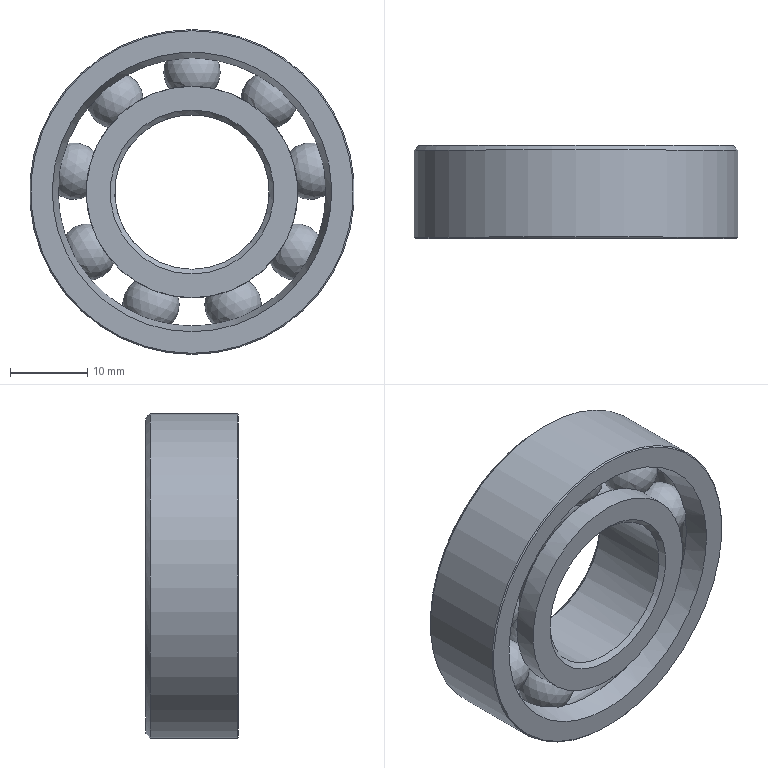Part | STEP file | 冲床-300配套压波_id814_x_t | 1 solid | 41 faces | box 42 x 12 x 42 mm | volume 8804 mm3 | torus 18 | sphere 9 | cylinder 5 | cone 5 | plane 4 | commonest cylinder face diameters 27.334 x2 20 x1 34.666 x1 42 x1